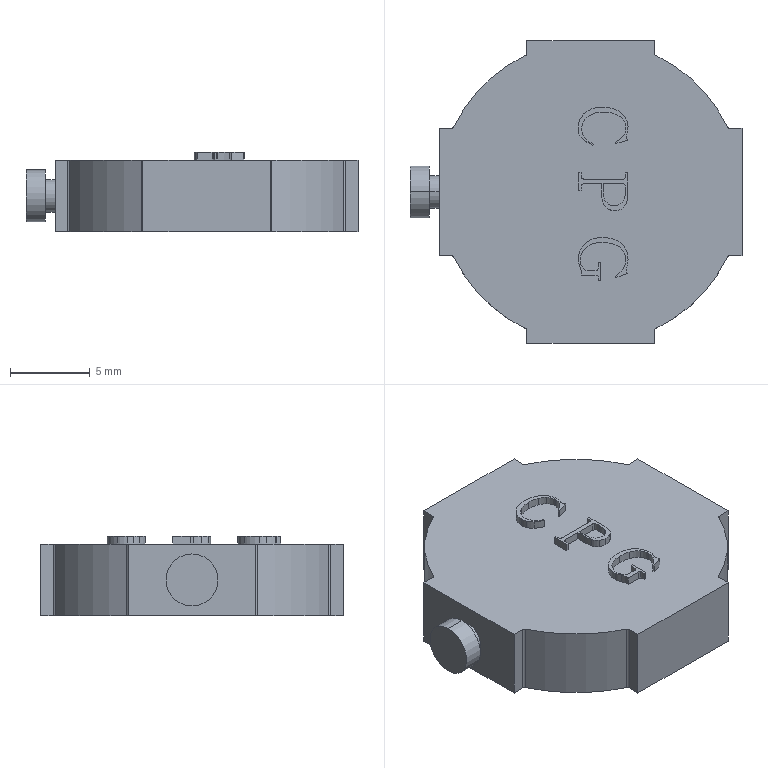Part | SolidWorks | features BaseBody 1 | 1 solid | 121 faces | box 20.838 x 19 x 5 mm | volume 1332 mm3 | spline 65 | plane 40 | cylinder 16 | commonest cylinder face diameters 0.3 x8 19 x4 2.039 x2 3.262 x2